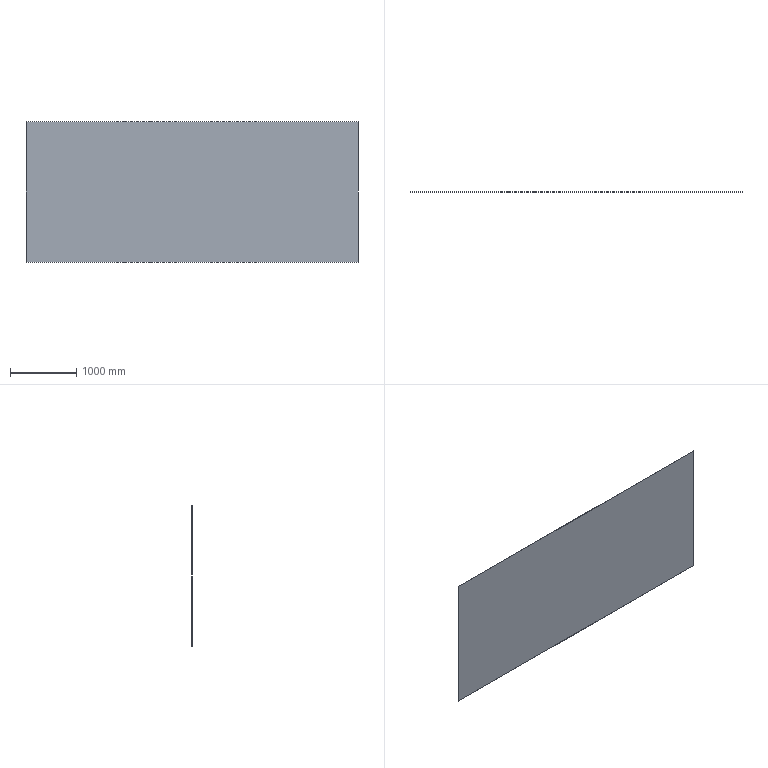Part | SolidWorks | features Extrusion 1 | 1 solid | 6 faces | box 5020 x 3 x 2120 mm | volume 31927200 mm3 | plane 6
STEP:
#1=CARTESIAN_POINT('',(2510.,0.,1060.));
#2=VERTEX_POINT('',#1);
#3=CARTESIAN_POINT('',(2510.,0.,-1060.));
#4=VERTEX_POINT('',#3);
#5=CARTESIAN_POINT('',(2510.,0.,1060.));
#6=DIRECTION('',(0.,0.,-1.));
#7=VECTOR('',#6,1000.);
#8=LINE('',#5,#7);
#9=EDGE_CURVE('',#2,#4,#8,.T.);
#10=ORIENTED_EDGE('',*,*,#9,.T.);
#11=CARTESIAN_POINT('',(2510.,3.,-1060.));
#12=VERTEX_POINT('',#11);
#13=CARTESIAN_POINT('',(2510.,3.,-1060.));
#14=DIRECTION('',(0.,-1.,0.));
#15=VECTOR('',#14,1000.);
#16=LINE('',#13,#15);
#17=EDGE_CURVE('',#12,#4,#16,.T.);
#18=ORIENTED_EDGE('',*,*,#17,.F.);
#19=CARTESIAN_POINT('',(2510.,3.,1060.));
#20=VERTEX_POINT('',#19);
#21=CARTESIAN_POINT('',(2510.,3.,1060.));
#22=DIRECTION('',(0.,0.,-1.));
#23=VECTOR('',#22,1000.);
#24=LINE('',#21,#23);
#25=EDGE_CURVE('',#20,#12,#24,.T.);
#26=ORIENTED_EDGE('',*,*,#25,.F.);
#27=CARTESIAN_POINT('',(2510.,3.,1060.));
#28=DIRECTION('',(0.,-1.,0.));
#29=VECTOR('',#28,1000.);
#30=LINE('',#27,#29);
#31=EDGE_CURVE('',#20,#2,#30,.T.);
#32=ORIENTED_EDGE('',*,*,#31,.T.);
#33=EDGE_LOOP('',(#10,#18,#26,#32));
#34=FACE_OUTER_BOUND('',#33,.T.);
#35=CARTESIAN_POINT('',(2510.,3.,1060.));
#36=DIRECTION('',(-1.,0.,0.));
#37=DIRECTION('',(0.,0.,1.));
#38=AXIS2_PLACEMENT_3D('',#35,#36,#37);
#39=PLANE('',#38);
#40=ADVANCED_FACE('',(#34),#39,.F.);
#41=CARTESIAN_POINT('',(-2510.,0.,-1060.));
#42=VERTEX_POINT('',#41);
#43=CARTESIAN_POINT('',(-2510.,0.,-1060.));
#44=DIRECTION('',(-1.,0.,0.));
#45=VECTOR('',#44,1000.);
#46=LINE('',#43,#45);
#47=EDGE_CURVE('',#4,#42,#46,.T.);
#48=ORIENTED_EDGE('',*,*,#47,.T.);
#49=CARTESIAN_POINT('',(-2510.,3.,-1060.));
#50=VERTEX_POINT('',#49);
#51=CARTESIAN_POINT('',(-2510.,3.,-1060.));
#52=DIRECTION('',(0.,-1.,0.));
#53=VECTOR('',#52,1000.);
#54=LINE('',#51,#53);
#55=EDGE_CURVE('',#50,#42,#54,.T.);
#56=ORIENTED_EDGE('',*,*,#55,.F.);
#57=CARTESIAN_POINT('',(-2510.,3.,-1060.));
#58=DIRECTION('',(-1.,0.,0.));
#59=VECTOR('',#58,1000.);
#60=LINE('',#57,#59);
#61=EDGE_CURVE('',#12,#50,#60,.T.);
#62=ORIENTED_EDGE('',*,*,#61,.F.);
#63=ORIENTED_EDGE('',*,*,#17,.T.);
#64=EDGE_LOOP('',(#48,#56,#62,#63));
#65=FACE_OUTER_BOUND('',#64,.T.);
#66=CARTESIAN_POINT('',(-2510.,3.,-1060.));
#67=DIRECTION('',(0.,0.,1.));
#68=DIRECTION('',(1.,0.,0.));
#69=AXIS2_PLACEMENT_3D('',#66,#67,#68);
#70=PLANE('',#69);
#71=ADVANCED_FACE('',(#65),#70,.F.);
#72=CARTESIAN_POINT('',(-2510.,0.,1060.));
#73=VERTEX_POINT('',#72);
#74=CARTESIAN_POINT('',(-2510.,0.,1060.));
#75=DIRECTION('',(0.,0.,1.));
#76=VECTOR('',#75,1000.);
#77=LINE('',#74,#76);
#78=EDGE_CURVE('',#42,#73,#77,.T.);
#79=ORIENTED_EDGE('',*,*,#78,.T.);
#80=CARTESIAN_POINT('',(-2510.,3.,1060.));
#81=VERTEX_POINT('',#80);
#82=CARTESIAN_POINT('',(-2510.,3.,1060.));
#83=DIRECTION('',(0.,-1.,0.));
#84=VECTOR('',#83,1000.);
#85=LINE('',#82,#84);
#86=EDGE_CURVE('',#81,#73,#85,.T.);
#87=ORIENTED_EDGE('',*,*,#86,.F.);
#88=CARTESIAN_POINT('',(-2510.,3.,1060.));
#89=DIRECTION('',(0.,0.,1.));
#90=VECTOR('',#89,1000.);
#91=LINE('',#88,#90);
#92=EDGE_CURVE('',#50,#81,#91,.T.);
#93=ORIENTED_EDGE('',*,*,#92,.F.);
#94=ORIENTED_EDGE('',*,*,#55,.T.);
#95=EDGE_LOOP('',(#79,#87,#93,#94));
#96=FACE_OUTER_BOUND('',#95,.T.);
#97=CARTESIAN_POINT('',(-2510.,3.,1060.));
#98=DIRECTION('',(1.,0.,0.));
#99=DIRECTION('',(0.,0.,-1.));
#100=AXIS2_PLACEMENT_3D('',#97,#98,#99);
#101=PLANE('',#100);
#102=ADVANCED_FACE('',(#96),#101,.F.);
#103=CARTESIAN_POINT('',(-2510.,0.,1060.));
#104=DIRECTION('',(1.,0.,0.));
#105=VECTOR('',#104,1000.);
#106=LINE('',#103,#105);
#107=EDGE_CURVE('',#73,#2,#106,.T.);
#108=ORIENTED_EDGE('',*,*,#107,.T.);
#109=ORIENTED_EDGE('',*,*,#31,.F.);
#110=CARTESIAN_POINT('',(-2510.,3.,1060.));
#111=DIRECTION('',(1.,0.,0.));
#112=VECTOR('',#111,1000.);
#113=LINE('',#110,#112);
#114=EDGE_CURVE('',#81,#20,#113,.T.);
#115=ORIENTED_EDGE('',*,*,#114,.F.);
#116=ORIENTED_EDGE('',*,*,#86,.T.);
#117=EDGE_LOOP('',(#108,#109,#115,#116));
#118=FACE_OUTER_BOUND('',#117,.T.);
#119=CARTESIAN_POINT('',(-2510.,3.,1060.));
#120=DIRECTION('',(0.,0.,-1.));
#121=DIRECTION('',(-1.,0.,0.));
#122=AXIS2_PLACEMENT_3D('',#119,#120,#121);
#123=PLANE('',#122);
#124=ADVANCED_FACE('',(#118),#123,.F.);
#125=ORIENTED_EDGE('',*,*,#25,.T.);
#126=ORIENTED_EDGE('',*,*,#61,.T.);
#127=ORIENTED_EDGE('',*,*,#92,.T.);
#128=ORIENTED_EDGE('',*,*,#114,.T.);
#129=EDGE_LOOP('',(#125,#126,#127,#128));
#130=FACE_OUTER_BOUND('',#129,.T.);
#131=CARTESIAN_POINT('',(0.,3.,0.));
#132=DIRECTION('',(0.,-1.,0.));
#133=DIRECTION('',(0.,0.,-1.));
#134=AXIS2_PLACEMENT_3D('',#131,#132,#133);
#135=PLANE('',#134);
#136=ADVANCED_FACE('',(#130),#135,.F.);
#137=ORIENTED_EDGE('',*,*,#9,.F.);
#138=ORIENTED_EDGE('',*,*,#107,.F.);
#139=ORIENTED_EDGE('',*,*,#78,.F.);
#140=ORIENTED_EDGE('',*,*,#47,.F.);
#141=EDGE_LOOP('',(#137,#138,#139,#140));
#142=FACE_OUTER_BOUND('',#141,.T.);
#143=CARTESIAN_POINT('',(0.,0.,0.));
#144=DIRECTION('',(0.,-1.,0.));
#145=DIRECTION('',(0.,0.,-1.));
#146=AXIS2_PLACEMENT_3D('',#143,#144,#145);
#147=PLANE('',#146);
#148=ADVANCED_FACE('',(#142),#147,.T.);
#149=CLOSED_SHELL('',(#40,#71,#102,#124,#136,#148));
#150=MANIFOLD_SOLID_BREP('',#149);
#151=CARTESIAN_POINT('',(0.,0.,0.));
#152=DIRECTION('',(0.,0.,1.));
#153=DIRECTION('',(1.,0.,0.));
#154=AXIS2_PLACEMENT_3D('',#151,#152,#153);
#155=(LENGTH_UNIT()NAMED_UNIT(*)SI_UNIT(.MILLI.,.METRE.));
#156=UNCERTAINTY_MEASURE_WITH_UNIT(LENGTH_MEASURE(0.00001),#155,'','');
#157=(NAMED_UNIT(*)PLANE_ANGLE_UNIT()SI_UNIT($,.RADIAN.));
#158=(NAMED_UNIT(*)SI_UNIT($,.STERADIAN.)SOLID_ANGLE_UNIT());
#159=(GEOMETRIC_REPRESENTATION_CONTEXT(3)GLOBAL_UNCERTAINTY_ASSIGNED_CONTEXT((#156))GLOBAL_UNIT_ASSIGNED_CONTEXT((#155,#157,#158))REPRESENTATION_CONTEXT('',''));
#160=ADVANCED_BREP_SHAPE_REPRESENTATION('',(#150,#154),#159);